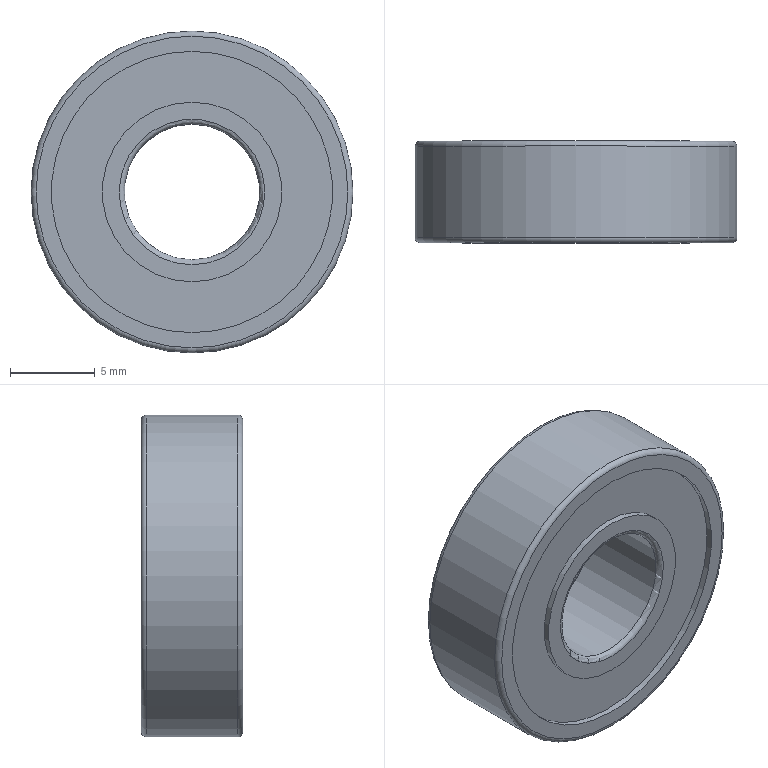Part | NX | features Bearing_5003_021_C-BGHA698ZZ-20 2 | 1 solid | 16 faces | box 19 x 6 x 19 mm | volume 1304 mm3 | plane 6 | cylinder 6 | torus 4 | commonest cylinder face diameters 10.6 x2 16.6 x2 8 x1 19 x1
STEP:
#1=CARTESIAN_POINT('',(213.825,-598.3,-114.5));
#2=VERTEX_POINT('',#1);
#3=CARTESIAN_POINT('',(213.825,-598.3,-110.5));
#4=DIRECTION('',(0.,-1.,0.));
#5=DIRECTION('',(0.,0.,-1.));
#6=AXIS2_PLACEMENT_3D('',#3,#4,#5);
#7=CIRCLE('',#6,4.);
#8=EDGE_CURVE('',#2,#2,#7,.T.);
#9=ORIENTED_EDGE('',*,*,#8,.F.);
#10=EDGE_LOOP('',(#9));
#11=FACE_BOUND('',#10,.T.);
#12=CARTESIAN_POINT('',(213.825,-598.6,-114.8));
#13=VERTEX_POINT('',#12);
#14=CARTESIAN_POINT('',(213.825,-598.6,-110.5));
#15=DIRECTION('',(0.,-1.,0.));
#16=DIRECTION('',(0.,0.,-1.));
#17=AXIS2_PLACEMENT_3D('',#14,#15,#16);
#18=CIRCLE('',#17,4.3);
#19=EDGE_CURVE('',#13,#13,#18,.T.);
#20=ORIENTED_EDGE('',*,*,#19,.T.);
#21=EDGE_LOOP('',(#20));
#22=FACE_BOUND('',#21,.T.);
#23=CARTESIAN_POINT('',(213.825,-598.3,-110.5));
#24=DIRECTION('',(0.,-1.,0.));
#25=DIRECTION('',(0.,0.,-1.));
#26=AXIS2_PLACEMENT_3D('',#23,#24,#25);
#27=TOROIDAL_SURFACE('',#26,4.3,0.3);
#28=ADVANCED_FACE('',(#11,#22),#27,.T.);
#29=ORIENTED_EDGE('',*,*,#19,.F.);
#30=EDGE_LOOP('',(#29));
#31=FACE_BOUND('',#30,.T.);
#32=CARTESIAN_POINT('',(213.825,-598.6,-115.8));
#33=VERTEX_POINT('',#32);
#34=CARTESIAN_POINT('',(213.825,-598.6,-110.5));
#35=DIRECTION('',(0.,-1.,0.));
#36=DIRECTION('',(0.,0.,-1.));
#37=AXIS2_PLACEMENT_3D('',#34,#35,#36);
#38=CIRCLE('',#37,5.3);
#39=EDGE_CURVE('',#33,#33,#38,.T.);
#40=ORIENTED_EDGE('',*,*,#39,.T.);
#41=EDGE_LOOP('',(#40));
#42=FACE_BOUND('',#41,.T.);
#43=CARTESIAN_POINT('',(219.125,-598.6,-110.5));
#44=DIRECTION('',(0.,1.,0.));
#45=DIRECTION('',(0.,0.,1.));
#46=AXIS2_PLACEMENT_3D('',#43,#44,#45);
#47=PLANE('',#46);
#48=ADVANCED_FACE('',(#31,#42),#47,.F.);
#49=ORIENTED_EDGE('',*,*,#39,.F.);
#50=EDGE_LOOP('',(#49));
#51=FACE_BOUND('',#50,.T.);
#52=CARTESIAN_POINT('',(213.825,-598.24,-115.8));
#53=VERTEX_POINT('',#52);
#54=CARTESIAN_POINT('',(213.825,-598.24,-110.5));
#55=DIRECTION('',(0.,-1.,0.));
#56=DIRECTION('',(0.,0.,-1.));
#57=AXIS2_PLACEMENT_3D('',#54,#55,#56);
#58=CIRCLE('',#57,5.3);
#59=EDGE_CURVE('',#53,#53,#58,.T.);
#60=ORIENTED_EDGE('',*,*,#59,.T.);
#61=EDGE_LOOP('',(#60));
#62=FACE_BOUND('',#61,.T.);
#63=CARTESIAN_POINT('',(213.825,-605.95,-110.5));
#64=DIRECTION('',(0.,-1.,0.));
#65=DIRECTION('',(0.,0.,-1.));
#66=AXIS2_PLACEMENT_3D('',#63,#64,#65);
#67=CYLINDRICAL_SURFACE('',#66,5.3);
#68=ADVANCED_FACE('',(#51,#62),#67,.T.);
#69=ORIENTED_EDGE('',*,*,#59,.F.);
#70=EDGE_LOOP('',(#69));
#71=FACE_BOUND('',#70,.T.);
#72=CARTESIAN_POINT('',(213.825,-598.24,-118.8));
#73=VERTEX_POINT('',#72);
#74=CARTESIAN_POINT('',(213.825,-598.24,-110.5));
#75=DIRECTION('',(0.,-1.,0.));
#76=DIRECTION('',(0.,0.,-1.));
#77=AXIS2_PLACEMENT_3D('',#74,#75,#76);
#78=CIRCLE('',#77,8.3);
#79=EDGE_CURVE('',#73,#73,#78,.T.);
#80=ORIENTED_EDGE('',*,*,#79,.T.);
#81=EDGE_LOOP('',(#80));
#82=FACE_BOUND('',#81,.T.);
#83=CARTESIAN_POINT('',(222.125,-598.24,-110.5));
#84=DIRECTION('',(0.,1.,0.));
#85=DIRECTION('',(0.,0.,1.));
#86=AXIS2_PLACEMENT_3D('',#83,#84,#85);
#87=PLANE('',#86);
#88=ADVANCED_FACE('',(#71,#82),#87,.F.);
#89=ORIENTED_EDGE('',*,*,#79,.F.);
#90=EDGE_LOOP('',(#89));
#91=FACE_BOUND('',#90,.T.);
#92=CARTESIAN_POINT('',(213.825,-598.6,-118.8));
#93=VERTEX_POINT('',#92);
#94=CARTESIAN_POINT('',(213.825,-598.6,-110.5));
#95=DIRECTION('',(0.,-1.,0.));
#96=DIRECTION('',(0.,0.,-1.));
#97=AXIS2_PLACEMENT_3D('',#94,#95,#96);
#98=CIRCLE('',#97,8.3);
#99=EDGE_CURVE('',#93,#93,#98,.T.);
#100=ORIENTED_EDGE('',*,*,#99,.T.);
#101=EDGE_LOOP('',(#100));
#102=FACE_BOUND('',#101,.T.);
#103=CARTESIAN_POINT('',(213.825,-605.95,-110.5));
#104=DIRECTION('',(0.,-1.,0.));
#105=DIRECTION('',(0.,0.,-1.));
#106=AXIS2_PLACEMENT_3D('',#103,#104,#105);
#107=CYLINDRICAL_SURFACE('',#106,8.3);
#108=ADVANCED_FACE('',(#91,#102),#107,.F.);
#109=ORIENTED_EDGE('',*,*,#99,.F.);
#110=EDGE_LOOP('',(#109));
#111=FACE_BOUND('',#110,.T.);
#112=CARTESIAN_POINT('',(213.825,-598.6,-119.7));
#113=VERTEX_POINT('',#112);
#114=CARTESIAN_POINT('',(213.825,-598.6,-110.5));
#115=DIRECTION('',(0.,-1.,0.));
#116=DIRECTION('',(0.,0.,-1.));
#117=AXIS2_PLACEMENT_3D('',#114,#115,#116);
#118=CIRCLE('',#117,9.2);
#119=EDGE_CURVE('',#113,#113,#118,.T.);
#120=ORIENTED_EDGE('',*,*,#119,.T.);
#121=EDGE_LOOP('',(#120));
#122=FACE_BOUND('',#121,.T.);
#123=CARTESIAN_POINT('',(223.025,-598.6,-110.5));
#124=DIRECTION('',(0.,1.,0.));
#125=DIRECTION('',(0.,0.,1.));
#126=AXIS2_PLACEMENT_3D('',#123,#124,#125);
#127=PLANE('',#126);
#128=ADVANCED_FACE('',(#111,#122),#127,.F.);
#129=ORIENTED_EDGE('',*,*,#119,.F.);
#130=EDGE_LOOP('',(#129));
#131=FACE_BOUND('',#130,.T.);
#132=CARTESIAN_POINT('',(213.825,-598.3,-120.));
#133=VERTEX_POINT('',#132);
#134=CARTESIAN_POINT('',(213.825,-598.3,-110.5));
#135=DIRECTION('',(0.,-1.,0.));
#136=DIRECTION('',(0.,0.,-1.));
#137=AXIS2_PLACEMENT_3D('',#134,#135,#136);
#138=CIRCLE('',#137,9.5);
#139=EDGE_CURVE('',#133,#133,#138,.T.);
#140=ORIENTED_EDGE('',*,*,#139,.T.);
#141=EDGE_LOOP('',(#140));
#142=FACE_BOUND('',#141,.T.);
#143=CARTESIAN_POINT('',(213.825,-598.3,-110.5));
#144=DIRECTION('',(0.,-1.,0.));
#145=DIRECTION('',(0.,0.,-1.));
#146=AXIS2_PLACEMENT_3D('',#143,#144,#145);
#147=TOROIDAL_SURFACE('',#146,9.2,0.3);
#148=ADVANCED_FACE('',(#131,#142),#147,.T.);
#149=ORIENTED_EDGE('',*,*,#139,.F.);
#150=EDGE_LOOP('',(#149));
#151=FACE_BOUND('',#150,.T.);
#152=CARTESIAN_POINT('',(213.825,-592.9,-120.));
#153=VERTEX_POINT('',#152);
#154=CARTESIAN_POINT('',(213.825,-592.9,-110.5));
#155=DIRECTION('',(0.,-1.,0.));
#156=DIRECTION('',(0.,0.,-1.));
#157=AXIS2_PLACEMENT_3D('',#154,#155,#156);
#158=CIRCLE('',#157,9.5);
#159=EDGE_CURVE('',#153,#153,#158,.T.);
#160=ORIENTED_EDGE('',*,*,#159,.T.);
#161=EDGE_LOOP('',(#160));
#162=FACE_BOUND('',#161,.T.);
#163=CARTESIAN_POINT('',(213.825,-605.95,-110.5));
#164=DIRECTION('',(0.,-1.,0.));
#165=DIRECTION('',(0.,0.,-1.));
#166=AXIS2_PLACEMENT_3D('',#163,#164,#165);
#167=CYLINDRICAL_SURFACE('',#166,9.5);
#168=ADVANCED_FACE('',(#151,#162),#167,.T.);
#169=ORIENTED_EDGE('',*,*,#159,.F.);
#170=EDGE_LOOP('',(#169));
#171=FACE_BOUND('',#170,.T.);
#172=CARTESIAN_POINT('',(213.825,-592.6,-119.7));
#173=VERTEX_POINT('',#172);
#174=CARTESIAN_POINT('',(213.825,-592.6,-110.5));
#175=DIRECTION('',(0.,-1.,0.));
#176=DIRECTION('',(0.,0.,-1.));
#177=AXIS2_PLACEMENT_3D('',#174,#175,#176);
#178=CIRCLE('',#177,9.2);
#179=EDGE_CURVE('',#173,#173,#178,.T.);
#180=ORIENTED_EDGE('',*,*,#179,.T.);
#181=EDGE_LOOP('',(#180));
#182=FACE_BOUND('',#181,.T.);
#183=CARTESIAN_POINT('',(213.825,-592.9,-110.5));
#184=DIRECTION('',(0.,-1.,0.));
#185=DIRECTION('',(0.,0.,-1.));
#186=AXIS2_PLACEMENT_3D('',#183,#184,#185);
#187=TOROIDAL_SURFACE('',#186,9.2,0.3);
#188=ADVANCED_FACE('',(#171,#182),#187,.T.);
#189=ORIENTED_EDGE('',*,*,#179,.F.);
#190=EDGE_LOOP('',(#189));
#191=FACE_BOUND('',#190,.T.);
#192=CARTESIAN_POINT('',(213.825,-592.6,-118.8));
#193=VERTEX_POINT('',#192);
#194=CARTESIAN_POINT('',(213.825,-592.6,-110.5));
#195=DIRECTION('',(0.,-1.,0.));
#196=DIRECTION('',(0.,0.,-1.));
#197=AXIS2_PLACEMENT_3D('',#194,#195,#196);
#198=CIRCLE('',#197,8.3);
#199=EDGE_CURVE('',#193,#193,#198,.T.);
#200=ORIENTED_EDGE('',*,*,#199,.T.);
#201=EDGE_LOOP('',(#200));
#202=FACE_BOUND('',#201,.T.);
#203=CARTESIAN_POINT('',(223.025,-592.6,-110.5));
#204=DIRECTION('',(0.,-1.,0.));
#205=DIRECTION('',(0.,0.,-1.));
#206=AXIS2_PLACEMENT_3D('',#203,#204,#205);
#207=PLANE('',#206);
#208=ADVANCED_FACE('',(#191,#202),#207,.F.);
#209=ORIENTED_EDGE('',*,*,#199,.F.);
#210=EDGE_LOOP('',(#209));
#211=FACE_BOUND('',#210,.T.);
#212=CARTESIAN_POINT('',(213.825,-592.96,-118.8));
#213=VERTEX_POINT('',#212);
#214=CARTESIAN_POINT('',(213.825,-592.96,-110.5));
#215=DIRECTION('',(0.,-1.,0.));
#216=DIRECTION('',(0.,0.,-1.));
#217=AXIS2_PLACEMENT_3D('',#214,#215,#216);
#218=CIRCLE('',#217,8.3);
#219=EDGE_CURVE('',#213,#213,#218,.T.);
#220=ORIENTED_EDGE('',*,*,#219,.T.);
#221=EDGE_LOOP('',(#220));
#222=FACE_BOUND('',#221,.T.);
#223=CARTESIAN_POINT('',(213.825,-605.95,-110.5));
#224=DIRECTION('',(0.,-1.,0.));
#225=DIRECTION('',(0.,0.,-1.));
#226=AXIS2_PLACEMENT_3D('',#223,#224,#225);
#227=CYLINDRICAL_SURFACE('',#226,8.3);
#228=ADVANCED_FACE('',(#211,#222),#227,.F.);
#229=ORIENTED_EDGE('',*,*,#219,.F.);
#230=EDGE_LOOP('',(#229));
#231=FACE_BOUND('',#230,.T.);
#232=CARTESIAN_POINT('',(213.825,-592.96,-115.8));
#233=VERTEX_POINT('',#232);
#234=CARTESIAN_POINT('',(213.825,-592.96,-110.5));
#235=DIRECTION('',(0.,-1.,0.));
#236=DIRECTION('',(0.,0.,-1.));
#237=AXIS2_PLACEMENT_3D('',#234,#235,#236);
#238=CIRCLE('',#237,5.3);
#239=EDGE_CURVE('',#233,#233,#238,.T.);
#240=ORIENTED_EDGE('',*,*,#239,.T.);
#241=EDGE_LOOP('',(#240));
#242=FACE_BOUND('',#241,.T.);
#243=CARTESIAN_POINT('',(222.125,-592.96,-110.5));
#244=DIRECTION('',(0.,-1.,0.));
#245=DIRECTION('',(0.,0.,-1.));
#246=AXIS2_PLACEMENT_3D('',#243,#244,#245);
#247=PLANE('',#246);
#248=ADVANCED_FACE('',(#231,#242),#247,.F.);
#249=ORIENTED_EDGE('',*,*,#239,.F.);
#250=EDGE_LOOP('',(#249));
#251=FACE_BOUND('',#250,.T.);
#252=CARTESIAN_POINT('',(213.825,-592.6,-115.8));
#253=VERTEX_POINT('',#252);
#254=CARTESIAN_POINT('',(213.825,-592.6,-110.5));
#255=DIRECTION('',(0.,-1.,0.));
#256=DIRECTION('',(0.,0.,-1.));
#257=AXIS2_PLACEMENT_3D('',#254,#255,#256);
#258=CIRCLE('',#257,5.3);
#259=EDGE_CURVE('',#253,#253,#258,.T.);
#260=ORIENTED_EDGE('',*,*,#259,.T.);
#261=EDGE_LOOP('',(#260));
#262=FACE_BOUND('',#261,.T.);
#263=CARTESIAN_POINT('',(213.825,-605.95,-110.5));
#264=DIRECTION('',(0.,-1.,0.));
#265=DIRECTION('',(0.,0.,-1.));
#266=AXIS2_PLACEMENT_3D('',#263,#264,#265);
#267=CYLINDRICAL_SURFACE('',#266,5.3);
#268=ADVANCED_FACE('',(#251,#262),#267,.T.);
#269=ORIENTED_EDGE('',*,*,#259,.F.);
#270=EDGE_LOOP('',(#269));
#271=FACE_BOUND('',#270,.T.);
#272=CARTESIAN_POINT('',(213.825,-592.6,-114.8));
#273=VERTEX_POINT('',#272);
#274=CARTESIAN_POINT('',(213.825,-592.6,-110.5));
#275=DIRECTION('',(0.,-1.,0.));
#276=DIRECTION('',(0.,0.,-1.));
#277=AXIS2_PLACEMENT_3D('',#274,#275,#276);
#278=CIRCLE('',#277,4.3);
#279=EDGE_CURVE('',#273,#273,#278,.T.);
#280=ORIENTED_EDGE('',*,*,#279,.T.);
#281=EDGE_LOOP('',(#280));
#282=FACE_BOUND('',#281,.T.);
#283=CARTESIAN_POINT('',(219.125,-592.6,-110.5));
#284=DIRECTION('',(0.,-1.,0.));
#285=DIRECTION('',(0.,0.,-1.));
#286=AXIS2_PLACEMENT_3D('',#283,#284,#285);
#287=PLANE('',#286);
#288=ADVANCED_FACE('',(#271,#282),#287,.F.);
#289=ORIENTED_EDGE('',*,*,#279,.F.);
#290=EDGE_LOOP('',(#289));
#291=FACE_BOUND('',#290,.T.);
#292=CARTESIAN_POINT('',(213.825,-592.9,-114.5));
#293=VERTEX_POINT('',#292);
#294=CARTESIAN_POINT('',(213.825,-592.9,-110.5));
#295=DIRECTION('',(0.,-1.,0.));
#296=DIRECTION('',(0.,0.,-1.));
#297=AXIS2_PLACEMENT_3D('',#294,#295,#296);
#298=CIRCLE('',#297,4.);
#299=EDGE_CURVE('',#293,#293,#298,.T.);
#300=ORIENTED_EDGE('',*,*,#299,.T.);
#301=EDGE_LOOP('',(#300));
#302=FACE_BOUND('',#301,.T.);
#303=CARTESIAN_POINT('',(213.825,-592.9,-110.5));
#304=DIRECTION('',(0.,-1.,0.));
#305=DIRECTION('',(0.,0.,-1.));
#306=AXIS2_PLACEMENT_3D('',#303,#304,#305);
#307=TOROIDAL_SURFACE('',#306,4.3,0.3);
#308=ADVANCED_FACE('',(#291,#302),#307,.T.);
#309=ORIENTED_EDGE('',*,*,#299,.F.);
#310=EDGE_LOOP('',(#309));
#311=FACE_BOUND('',#310,.T.);
#312=ORIENTED_EDGE('',*,*,#8,.T.);
#313=EDGE_LOOP('',(#312));
#314=FACE_BOUND('',#313,.T.);
#315=CARTESIAN_POINT('',(213.825,-605.95,-110.5));
#316=DIRECTION('',(0.,-1.,0.));
#317=DIRECTION('',(0.,0.,-1.));
#318=AXIS2_PLACEMENT_3D('',#315,#316,#317);
#319=CYLINDRICAL_SURFACE('',#318,4.);
#320=ADVANCED_FACE('',(#311,#314),#319,.F.);
#321=CLOSED_SHELL('',(#28,#48,#68,#88,#108,#128,#148,#168,#188,#208,#228,#248,#268,#288,#308,#320));
#322=MANIFOLD_SOLID_BREP('',#321);
#323=(LENGTH_UNIT()NAMED_UNIT(*)SI_UNIT(.MILLI.,.METRE.));
#324=UNCERTAINTY_MEASURE_WITH_UNIT(LENGTH_MEASURE(0.00001),#323,'','');
#325=(NAMED_UNIT(*)PLANE_ANGLE_UNIT()SI_UNIT($,.RADIAN.));
#326=(NAMED_UNIT(*)SI_UNIT($,.STERADIAN.)SOLID_ANGLE_UNIT());
#327=(GEOMETRIC_REPRESENTATION_CONTEXT(3)GLOBAL_UNCERTAINTY_ASSIGNED_CONTEXT((#324))GLOBAL_UNIT_ASSIGNED_CONTEXT((#323,#325,#326))REPRESENTATION_CONTEXT('',''));
#328=ADVANCED_BREP_SHAPE_REPRESENTATION('',(#322),#327);